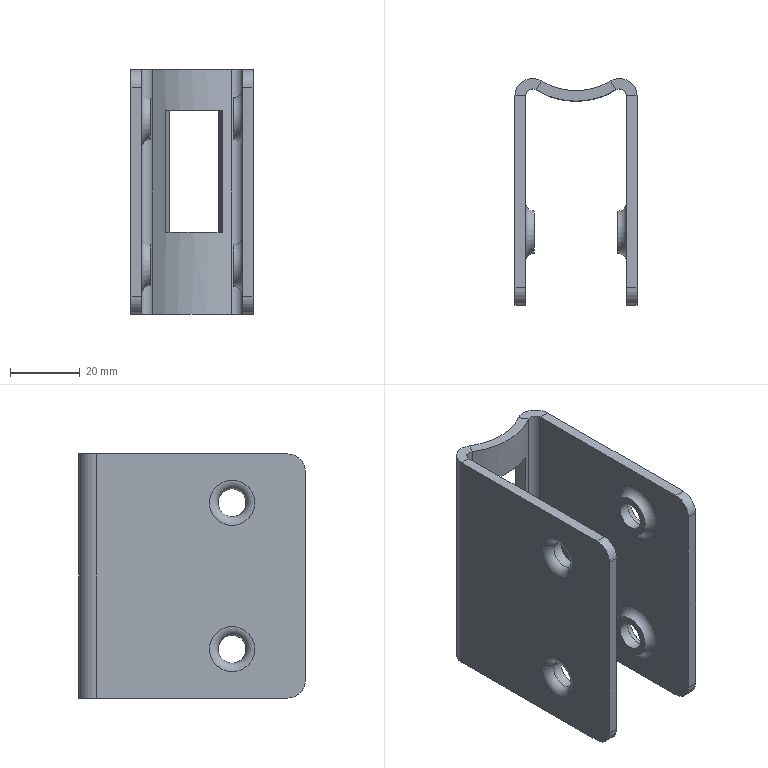Part | STEP file | PN_0011_default | 1 solid | 46 faces | box 35 x 65 x 70 mm | volume 31433 mm3 | plane 24 | cylinder 14 | torus 8 | commonest cylinder face diameters 10 x6 8 x4 4 x2 38.129 x1 44.129 x1